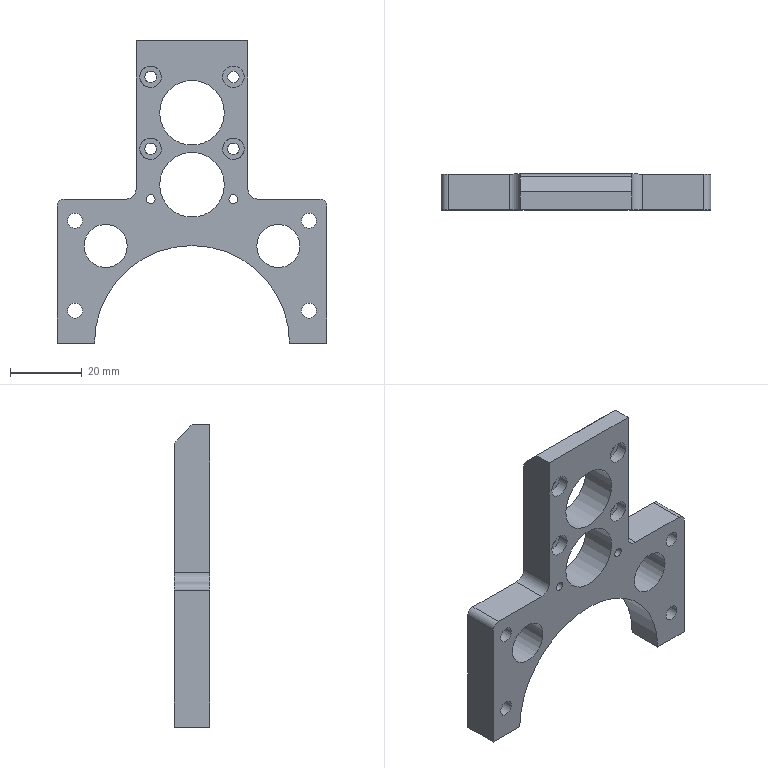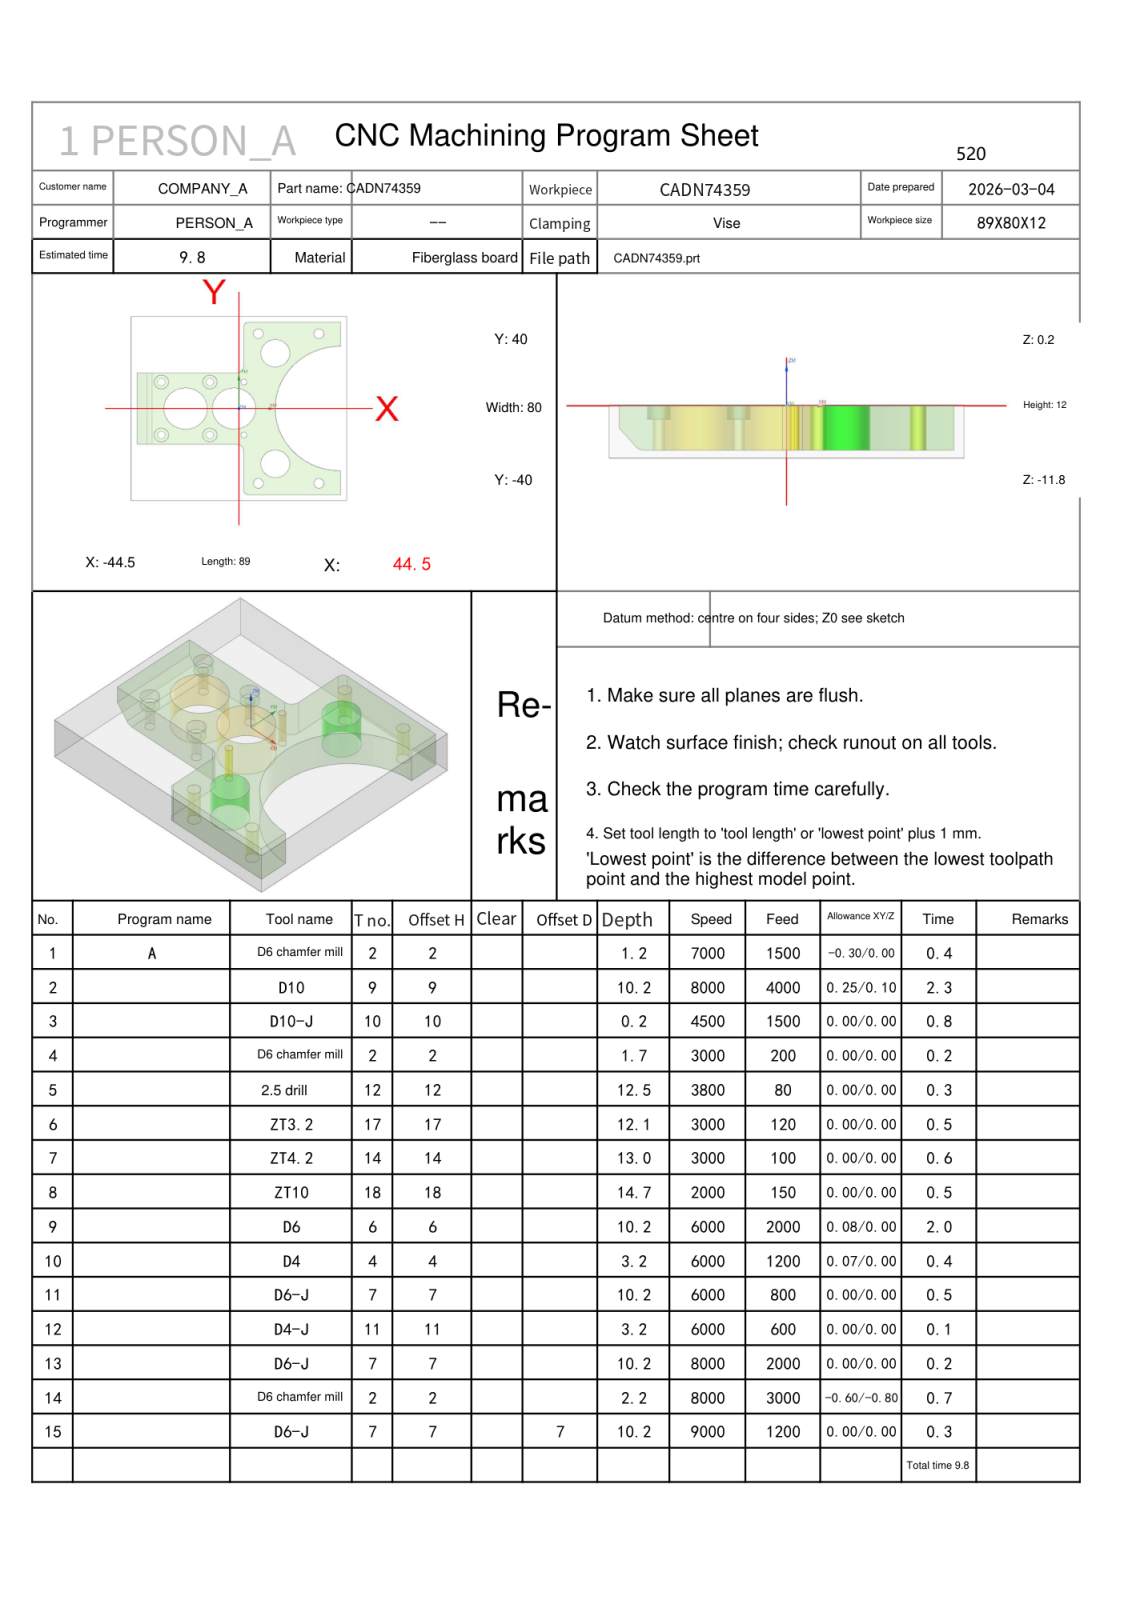NC program | NX | posted by the shop | part box 75 x 10 x 84 mm
Lines 1 to 167 of 4435:
%
O0001
(Machine time: 12.68 MIN)
(===Total Tool:11===)
(T2=D6 chamfer mill   D=6.   R=0.   D-  H02 Z=-2.   )
(T9=D10     D=10.  R=0.   D-  H09 Z=-10.  )
(T10=D10-J  D=10.  R=0.   D-  H10 Z=-0.   )
(T12=2.5 drill  D=2.5  DR_a=118 D-  H12 Z=-12.25)
(T17=ZT3.2  D=3.2  DR_a=120 D-  H17 Z=-11.92)
(T14=ZT4.2  D=4.2  DR_a=118 D-  H14 Z=-12.76)
(T18=ZT10   D=10.  DR_a=118 D-  H18 Z=-14.5 )
(T6=D6      D=6.   R=0.   D-  H06 Z=-10.  )
(T4=D4      D=4.   R=0.   D-  H04 Z=-3.   )
(T7=D6-J    D=6.   R=0.   D7  H07 Z=-10.  )
(T11=D4-J   D=4.   R=0.   D-  H11 Z=-3.   )
G80 G90 G17 G49 G40
G91 G28 Z0
M01
N1 T02 M06
(D6 chamfer mill  D=6. R=0. H=02 ce=-0.30 di=0.00)
G00 G90 G54 X1.3 Y25.884 M03 S7000
G43 H02 Z50.
M08
Z2.5
G01 Y35.5 Z-1. F1500.
G02 X4. Y38.2 I2.7 J0.0
G01 X41.7
G02 X42.7 Y37.2 I0.0 J-1.
G01 Y27.398
G02 X41.711 Y26.398 I-1. J0.0
G03 X15.6 Y0.0 I.289 J-26.398
X41.711 Y-26.398 I26.4 J0.0
G02 X42.7 Y-27.398 I-.011 J-1.
G01 Y-37.2
G02 X41.7 Y-38.2 I-1. J0.0
G01 X4.
G02 X1.3 Y-35.5 I0.0 J2.7
G01 Y-18.5
G03 X-1. Y-16.2 I-2.3 J0.0
G01 X-41.7
G02 X-42.7 Y-15.2 I0.0 J1.
G01 Y15.2
G02 X-41.7 Y16.2 I1. J0.0
G01 X-1.
G03 X1.3 Y18.5 I0.0 J2.3
G01 Y35.5
G02 X1.346 Y35.997 I2.7 J0.0
G01 Z1.5
G00 Z50.
G00 G90 X16.276 Y29.142 M03 S7000
Z50.
Z2.5
G01 X16.124 Y29.183 Z2.443 F1500.
X15.642 Y29.264 Z2.265
X15.155 Y29.301 Z2.087
X14.667 Y29.293 Z1.909
X14.181 Y29.239 Z1.732
X13.703 Y29.142 Z1.554
X13.235 Y29.001 Z1.376
X12.782 Y28.817 Z1.198
X12.349 Y28.593 Z1.021
X11.937 Y28.329 Z.843
X11.552 Y28.029 Z.665
X11.196 Y27.695 Z.487
X10.872 Y27.329 Z.309
X10.583 Y26.935 Z.132
X10.332 Y26.516 Z-.046
X10.12 Y26.076 Z-.224
X9.95 Y25.618 Z-.402
X9.822 Y25.147 Z-.58
X9.739 Y24.665 Z-.757
X9.7 Y24.178 Z-.935
Y24. Z-1.
G03 X15. Y18.7 I5.3 J0.0
X20.3 Y24. I0.0 J5.3
X15. Y29.3 I-5.3 J0.0
X9.7 Y24. I0.0 J-5.3
X9.724 Y23.501 I5.3 J0.0
G01 Z1.5
G00 Z50.
X-5.327 Y7.606
Z2.5
G01 X-5.877 Y7.342 Z2.278
X-6.42 Y7.029 Z2.05
X-6.938 Y6.675 Z1.821
X-7.428 Y6.283 Z1.593
X-7.887 Y5.855 Z1.365
X-8.312 Y5.394 Z1.136
X-8.702 Y4.902 Z.908
X-9.053 Y4.382 Z.68
X-9.363 Y3.837 Z.451
X-9.632 Y3.27 Z.223
X-9.857 Y2.684 Z-.005
X-10.037 Y2.083 Z-.234
X-10.172 Y1.47 Z-.462
X-10.259 Y.849 Z-.69
X-10.3 Y.223 Z-.919
Y0.0 Z-1.
G03 X-2. Y-8.3 I8.3 J0.0
X6.3 Y0.0 I0.0 J8.3
X-2. Y8.3 I-8.3 J0.0
X-10.3 Y0.0 I0.0 J-8.3
X-10.285 Y-.5 I8.3 J0.0
G01 Z1.5
G00 Z50.
X-25.327 Y7.606
Z2.5
G01 X-25.877 Y7.342 Z2.278
X-26.42 Y7.029 Z2.05
X-26.938 Y6.675 Z1.821
X-27.428 Y6.283 Z1.593
X-27.887 Y5.855 Z1.365
X-28.312 Y5.394 Z1.136
X-28.702 Y4.902 Z.908
X-29.053 Y4.382 Z.68
X-29.363 Y3.837 Z.451
X-29.632 Y3.27 Z.223
X-29.857 Y2.684 Z-.005
X-30.037 Y2.083 Z-.234
X-30.172 Y1.47 Z-.462
X-30.259 Y.849 Z-.69
X-30.3 Y.223 Z-.919
Y0.0 Z-1.
G03 X-22. Y-8.3 I8.3 J0.0
X-13.7 Y0.0 I0.0 J8.3
X-22. Y8.3 I-8.3 J0.0
X-30.3 Y0.0 I0.0 J-8.3
X-30.285 Y-.5 I8.3 J0.0
G01 Z1.5
G00 Z50.
X16.276 Y-18.858
Z2.5
G01 X16.124 Y-18.817 Z2.443
X15.642 Y-18.736 Z2.265
X15.155 Y-18.699 Z2.087
X14.667 Y-18.707 Z1.909
X14.181 Y-18.761 Z1.732
X13.703 Y-18.858 Z1.554
X13.235 Y-18.999 Z1.376
X12.782 Y-19.183 Z1.198
X12.349 Y-19.407 Z1.021
X11.937 Y-19.671 Z.843
X11.552 Y-19.971 Z.665
X11.196 Y-20.305 Z.487
X10.872 Y-20.671 Z.309
X10.583 Y-21.065 Z.132
X10.332 Y-21.484 Z-.046
X10.12 Y-21.924 Z-.224
X9.95 Y-22.382 Z-.402
X9.822 Y-22.853 Z-.58
X9.739 Y-23.335 Z-.757
X9.7 Y-23.822 Z-.935
Y-24. Z-1.
G03 X15. Y-29.3 I5.3 J0.0
X20.3 Y-24. I0.0 J5.3
X15. Y-18.7 I-5.3 J0.0
X9.7 Y-24. I0.0 J-5.3
X9.724 Y-24.499 I5.3 J0.0
G01 Z1.5
G00 Z50.
G91 G28 Z0.0
M05
M09
G91 G28 Z0.0
M01